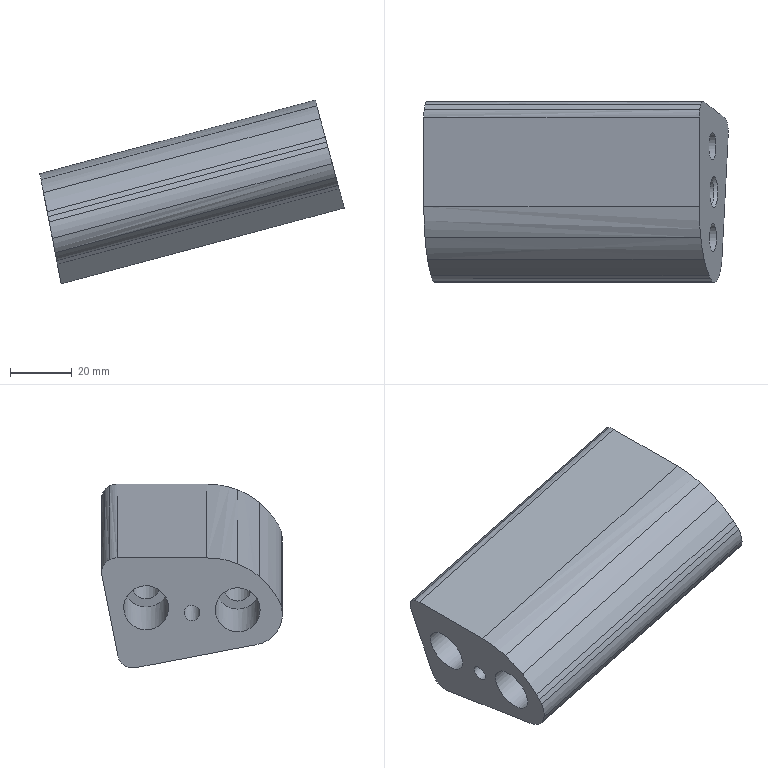Part | NX | features solid 2 | 1 solid | 31 faces | box 98.643 x 58.579 x 59.607 mm | volume 135213 mm3 | spline 16 | plane 8 | cylinder 6 | cone 1 | commonest cylinder face diameters 9.007 x2 14.508 x2 5.1 x1 8 x1
STEP:
#1=CARTESIAN_POINT('',(816.535,-85.556,-16.752));
#2=VERTEX_POINT('',#1);
#3=CARTESIAN_POINT('',(815.148,-85.584,-9.614));
#4=DIRECTION('',(0.9816,0.0002628,0.1908));
#5=DIRECTION('',(0.1908,0.003761,-0.9816));
#6=AXIS2_PLACEMENT_3D('',#3,#4,#5);
#7=ELLIPSE('',#6,7.272,7.254);
#8=EDGE_CURVE('',#2,#2,#7,.T.);
#9=ORIENTED_EDGE('',*,*,#8,.T.);
#10=EDGE_LOOP('',(#9));
#11=FACE_BOUND('',#10,.T.);
#12=CARTESIAN_POINT('',(816.396,-55.874,-16.077));
#13=VERTEX_POINT('',#12);
#14=CARTESIAN_POINT('',(815.009,-55.901,-8.939));
#15=DIRECTION('',(0.9816,0.0002628,0.1908));
#16=DIRECTION('',(0.1908,0.003761,-0.9816));
#17=AXIS2_PLACEMENT_3D('',#14,#15,#16);
#18=ELLIPSE('',#17,7.272,7.254);
#19=EDGE_CURVE('',#13,#13,#18,.T.);
#20=ORIENTED_EDGE('',*,*,#19,.T.);
#21=EDGE_LOOP('',(#20));
#22=FACE_BOUND('',#21,.T.);
#23=CARTESIAN_POINT('',(811.973,-44.117,6.663));
#24=VERTEX_POINT('',#23);
#25=CARTESIAN_POINT('',(811.863,-46.498,7.229));
#26=VERTEX_POINT('',#25);
#27=CARTESIAN_POINT('',(811.973,-44.117,6.663));
#28=CARTESIAN_POINT('',(811.9,-44.854,7.038));
#29=CARTESIAN_POINT('',(811.863,-45.668,7.229));
#30=CARTESIAN_POINT('',(811.863,-46.498,7.229));
#31=B_SPLINE_CURVE_WITH_KNOTS('',3,(#27,#28,#29,#30),.UNSPECIFIED.,.F.,.F.,(4,4),(0.,0.002457),.UNSPECIFIED.);
#32=EDGE_CURVE('',#24,#26,#31,.T.);
#33=ORIENTED_EDGE('',*,*,#32,.F.);
#34=CARTESIAN_POINT('',(812.277,-42.305,5.095));
#35=VERTEX_POINT('',#34);
#36=CARTESIAN_POINT('',(812.277,-42.305,5.095));
#37=CARTESIAN_POINT('',(812.148,-42.767,5.759));
#38=CARTESIAN_POINT('',(812.045,-43.389,6.293));
#39=CARTESIAN_POINT('',(811.973,-44.117,6.663));
#40=B_SPLINE_CURVE_WITH_KNOTS('',3,(#36,#37,#38,#39),.UNSPECIFIED.,.F.,.F.,(4,4),(0.,0.002422),.UNSPECIFIED.);
#41=EDGE_CURVE('',#35,#24,#40,.T.);
#42=ORIENTED_EDGE('',*,*,#41,.F.);
#43=CARTESIAN_POINT('',(812.6,-41.584,3.431));
#44=VERTEX_POINT('',#43);
#45=CARTESIAN_POINT('',(812.6,-41.584,3.431));
#46=CARTESIAN_POINT('',(812.483,-41.711,4.033));
#47=CARTESIAN_POINT('',(812.376,-41.952,4.587));
#48=CARTESIAN_POINT('',(812.277,-42.305,5.095));
#49=B_SPLINE_CURVE_WITH_KNOTS('',3,(#45,#46,#47,#48),.UNSPECIFIED.,.F.,.F.,(4,4),(0.,0.001842),.UNSPECIFIED.);
#50=EDGE_CURVE('',#44,#35,#49,.T.);
#51=ORIENTED_EDGE('',*,*,#50,.F.);
#52=CARTESIAN_POINT('',(812.953,-41.572,1.616));
#53=VERTEX_POINT('',#52);
#54=CARTESIAN_POINT('',(812.953,-41.572,1.616));
#55=CARTESIAN_POINT('',(812.835,-41.454,2.222));
#56=CARTESIAN_POINT('',(812.718,-41.457,2.827));
#57=CARTESIAN_POINT('',(812.6,-41.584,3.431));
#58=B_SPLINE_CURVE_WITH_KNOTS('',3,(#54,#55,#56,#57),.UNSPECIFIED.,.F.,.F.,(4,4),(0.,0.001849),.UNSPECIFIED.);
#59=EDGE_CURVE('',#53,#44,#58,.T.);
#60=ORIENTED_EDGE('',*,*,#59,.F.);
#61=CARTESIAN_POINT('',(814.349,-42.975,-5.566));
#62=VERTEX_POINT('',#61);
#63=CARTESIAN_POINT('',(814.349,-42.975,-5.566));
#64=CARTESIAN_POINT('',(813.884,-42.505,-3.172));
#65=CARTESIAN_POINT('',(813.419,-42.037,-0.7784));
#66=CARTESIAN_POINT('',(812.953,-41.572,1.616));
#67=B_SPLINE_CURVE_WITH_KNOTS('',3,(#63,#64,#65,#66),.UNSPECIFIED.,.F.,.F.,(4,4),(0.,0.007449),.UNSPECIFIED.);
#68=EDGE_CURVE('',#62,#53,#67,.T.);
#69=ORIENTED_EDGE('',*,*,#68,.F.);
#70=CARTESIAN_POINT('',(815.759,-44.406,-12.814));
#71=VERTEX_POINT('',#70);
#72=CARTESIAN_POINT('',(815.759,-44.406,-12.814));
#73=CARTESIAN_POINT('',(815.289,-43.926,-10.398));
#74=CARTESIAN_POINT('',(814.819,-43.45,-7.982));
#75=CARTESIAN_POINT('',(814.349,-42.975,-5.566));
#76=B_SPLINE_CURVE_WITH_KNOTS('',3,(#72,#73,#74,#75),.UNSPECIFIED.,.F.,.F.,(4,4),(0.,0.007522),.UNSPECIFIED.);
#77=EDGE_CURVE('',#71,#62,#76,.T.);
#78=ORIENTED_EDGE('',*,*,#77,.F.);
#79=CARTESIAN_POINT('',(818.03,-46.723,-24.494));
#80=VERTEX_POINT('',#79);
#81=CARTESIAN_POINT('',(813.97,-42.581,-3.616));
#82=DIRECTION('',(0.1873,-0.1911,-0.9635));
#83=VECTOR('',#82,1000.);
#84=LINE('',#81,#83);
#85=EDGE_CURVE('',#71,#80,#84,.T.);
#86=ORIENTED_EDGE('',*,*,#85,.T.);
#87=CARTESIAN_POINT('',(818.785,-52.586,-28.373));
#88=VERTEX_POINT('',#87);
#89=CARTESIAN_POINT('',(818.785,-52.586,-28.373));
#90=CARTESIAN_POINT('',(818.833,-51.29,-28.621));
#91=CARTESIAN_POINT('',(818.723,-48.542,-28.06));
#92=CARTESIAN_POINT('',(818.277,-46.975,-25.766));
#93=CARTESIAN_POINT('',(818.03,-46.723,-24.494));
#94=B_SPLINE_CURVE_WITH_KNOTS('',3,(#89,#90,#91,#92,#93),.UNSPECIFIED.,.F.,.F.,(4,1,4),(0.,0.003905,0.007811),.UNSPECIFIED.);
#95=EDGE_CURVE('',#88,#80,#94,.T.);
#96=ORIENTED_EDGE('',*,*,#95,.F.);
#97=CARTESIAN_POINT('',(817.556,-85.892,-22.005));
#98=VERTEX_POINT('',#97);
#99=CARTESIAN_POINT('',(826.533,157.396,-68.523));
#100=DIRECTION('',(0.03622,0.9816,-0.1877));
#101=VECTOR('',#100,1000.);
#102=LINE('',#99,#101);
#103=EDGE_CURVE('',#98,#88,#102,.T.);
#104=ORIENTED_EDGE('',*,*,#103,.F.);
#105=CARTESIAN_POINT('',(817.343,-91.803,-20.901));
#106=VERTEX_POINT('',#105);
#107=CARTESIAN_POINT('',(817.343,-91.803,-20.901));
#108=CARTESIAN_POINT('',(817.413,-89.831,-21.261));
#109=CARTESIAN_POINT('',(817.484,-87.86,-21.628));
#110=CARTESIAN_POINT('',(817.556,-85.892,-22.005));
#111=B_SPLINE_CURVE_WITH_KNOTS('',3,(#107,#108,#109,#110),.UNSPECIFIED.,.F.,.F.,(4,4),(0.,0.006017),.UNSPECIFIED.);
#112=EDGE_CURVE('',#106,#98,#111,.T.);
#113=ORIENTED_EDGE('',*,*,#112,.F.);
#114=CARTESIAN_POINT('',(816.845,-96.945,-18.332));
#115=VERTEX_POINT('',#114);
#116=CARTESIAN_POINT('',(816.845,-96.945,-18.332));
#117=CARTESIAN_POINT('',(817.103,-95.518,-19.658));
#118=CARTESIAN_POINT('',(817.276,-93.734,-20.549));
#119=CARTESIAN_POINT('',(817.343,-91.803,-20.901));
#120=B_SPLINE_CURVE_WITH_KNOTS('',3,(#116,#117,#118,#119),.UNSPECIFIED.,.F.,.F.,(4,4),(0.,0.005811),.UNSPECIFIED.);
#121=EDGE_CURVE('',#115,#106,#120,.T.);
#122=ORIENTED_EDGE('',*,*,#121,.F.);
#123=CARTESIAN_POINT('',(815.948,-99.734,-13.713));
#124=VERTEX_POINT('',#123);
#125=CARTESIAN_POINT('',(815.948,-99.734,-13.713));
#126=CARTESIAN_POINT('',(816.292,-99.26,-15.479));
#127=CARTESIAN_POINT('',(816.602,-98.295,-17.076));
#128=CARTESIAN_POINT('',(816.845,-96.945,-18.332));
#129=B_SPLINE_CURVE_WITH_KNOTS('',3,(#125,#126,#127,#128),.UNSPECIFIED.,.F.,.F.,(4,4),(0.,0.005502),.UNSPECIFIED.);
#130=EDGE_CURVE('',#124,#115,#129,.T.);
#131=ORIENTED_EDGE('',*,*,#130,.F.);
#132=CARTESIAN_POINT('',(814.903,-99.633,-8.337));
#133=VERTEX_POINT('',#132);
#134=CARTESIAN_POINT('',(815.948,-99.734,-13.713));
#135=CARTESIAN_POINT('',(815.605,-100.208,-11.945));
#136=CARTESIAN_POINT('',(815.244,-100.172,-10.087));
#137=CARTESIAN_POINT('',(814.903,-99.633,-8.337));
#138=B_SPLINE_CURVE_WITH_KNOTS('',3,(#134,#135,#136,#137),.UNSPECIFIED.,.F.,.F.,(4,4),(0.,0.00551),.UNSPECIFIED.);
#139=EDGE_CURVE('',#124,#133,#138,.T.);
#140=ORIENTED_EDGE('',*,*,#139,.T.);
#141=CARTESIAN_POINT('',(814.571,-98.902,-6.628));
#142=VERTEX_POINT('',#141);
#143=CARTESIAN_POINT('',(814.571,-98.902,-6.628));
#144=CARTESIAN_POINT('',(814.677,-99.207,-7.173));
#145=CARTESIAN_POINT('',(814.788,-99.451,-7.742));
#146=CARTESIAN_POINT('',(814.903,-99.633,-8.337));
#147=B_SPLINE_CURVE_WITH_KNOTS('',3,(#143,#144,#145,#146),.UNSPECIFIED.,.F.,.F.,(4,4),(0.,0.001887),.UNSPECIFIED.);
#148=EDGE_CURVE('',#142,#133,#147,.T.);
#149=ORIENTED_EDGE('',*,*,#148,.F.);
#150=CARTESIAN_POINT('',(814.258,-97.948,-5.022));
#151=VERTEX_POINT('',#150);
#152=CARTESIAN_POINT('',(814.258,-97.948,-5.022));
#153=CARTESIAN_POINT('',(814.361,-98.28,-5.549));
#154=CARTESIAN_POINT('',(814.465,-98.598,-6.085));
#155=CARTESIAN_POINT('',(814.571,-98.902,-6.628));
#156=B_SPLINE_CURVE_WITH_KNOTS('',3,(#152,#153,#154,#155),.UNSPECIFIED.,.F.,.F.,(4,4),(0.,0.001895),.UNSPECIFIED.);
#157=EDGE_CURVE('',#151,#142,#156,.T.);
#158=ORIENTED_EDGE('',*,*,#157,.F.);
#159=CARTESIAN_POINT('',(813.062,-92.585,1.127));
#160=VERTEX_POINT('',#159);
#161=CARTESIAN_POINT('',(813.062,-92.585,1.127));
#162=CARTESIAN_POINT('',(813.407,-94.699,-0.6484));
#163=CARTESIAN_POINT('',(813.807,-96.484,-2.701));
#164=CARTESIAN_POINT('',(814.258,-97.948,-5.022));
#165=B_SPLINE_CURVE_WITH_KNOTS('',3,(#161,#162,#163,#164),.UNSPECIFIED.,.F.,.F.,(4,4),(0.,0.008246),.UNSPECIFIED.);
#166=EDGE_CURVE('',#160,#151,#165,.T.);
#167=ORIENTED_EDGE('',*,*,#166,.F.);
#168=CARTESIAN_POINT('',(812.247,-85.562,5.309));
#169=VERTEX_POINT('',#168);
#170=CARTESIAN_POINT('',(812.247,-85.562,5.309));
#171=CARTESIAN_POINT('',(812.446,-88.136,4.29));
#172=CARTESIAN_POINT('',(812.717,-90.477,2.898));
#173=CARTESIAN_POINT('',(813.062,-92.585,1.127));
#174=B_SPLINE_CURVE_WITH_KNOTS('',3,(#170,#171,#172,#173),.UNSPECIFIED.,.F.,.F.,(4,4),(0.,0.008214),.UNSPECIFIED.);
#175=EDGE_CURVE('',#169,#160,#174,.T.);
#176=ORIENTED_EDGE('',*,*,#175,.F.);
#177=CARTESIAN_POINT('',(811.874,-75.541,7.214));
#178=VERTEX_POINT('',#177);
#179=CARTESIAN_POINT('',(811.874,-75.541,7.214));
#180=CARTESIAN_POINT('',(811.875,-79.006,7.212));
#181=CARTESIAN_POINT('',(811.999,-82.348,6.581));
#182=CARTESIAN_POINT('',(812.247,-85.562,5.309));
#183=B_SPLINE_CURVE_WITH_KNOTS('',3,(#179,#180,#181,#182),.UNSPECIFIED.,.F.,.F.,(4,4),(0.,0.01021),.UNSPECIFIED.);
#184=EDGE_CURVE('',#178,#169,#183,.T.);
#185=ORIENTED_EDGE('',*,*,#184,.F.);
#186=CARTESIAN_POINT('',(811.874,-75.571,7.214));
#187=DIRECTION('',(-0.0003677,1.,0.000514));
#188=VECTOR('',#187,1000.);
#189=LINE('',#186,#188);
#190=EDGE_CURVE('',#178,#26,#189,.T.);
#191=ORIENTED_EDGE('',*,*,#190,.T.);
#192=EDGE_LOOP('',(#33,#42,#51,#60,#69,#78,#86,#96,#104,#113,#122,#131,#140,#149,#158,#167,#176,#185,#191));
#193=FACE_BOUND('',#192,.T.);
#194=CARTESIAN_POINT('',(814.852,-70.813,-8.111));
#195=VERTEX_POINT('',#194);
#196=CARTESIAN_POINT('',(815.339,-70.804,-10.62));
#197=DIRECTION('',(0.9816,0.0002628,0.1908));
#198=DIRECTION('',(-0.1908,-0.003761,0.9816));
#199=AXIS2_PLACEMENT_3D('',#196,#197,#198);
#200=ELLIPSE('',#199,2.556,2.55);
#201=EDGE_CURVE('',#195,#195,#200,.F.);
#202=ORIENTED_EDGE('',*,*,#201,.F.);
#203=EDGE_LOOP('',(#202));
#204=FACE_BOUND('',#203,.T.);
#205=CARTESIAN_POINT('',(825.905,158.037,-65.289));
#206=DIRECTION('',(0.9816,0.0002628,0.1908));
#207=DIRECTION('',(-0.1908,0.001526,0.9816));
#208=AXIS2_PLACEMENT_3D('',#205,#206,#207);
#209=PLANE('',#208);
#210=ADVANCED_FACE('',(#11,#22,#193,#204),#209,.F.);
#211=CARTESIAN_POINT('',(907.109,-70.804,8.793));
#212=VERTEX_POINT('',#211);
#213=CARTESIAN_POINT('',(905.814,-70.804,13.623));
#214=DIRECTION('',(0.9659,-0.000000134,0.2588));
#215=DIRECTION('',(0.2588,0.,-0.9659));
#216=AXIS2_PLACEMENT_3D('',#213,#214,#215);
#217=CIRCLE('',#216,5.);
#218=EDGE_CURVE('',#212,#212,#217,.F.);
#219=ORIENTED_EDGE('',*,*,#218,.T.);
#220=EDGE_LOOP('',(#219));
#221=FACE_BOUND('',#220,.T.);
#222=CARTESIAN_POINT('',(904.207,-55.901,19.624));
#223=VERTEX_POINT('',#222);
#224=CARTESIAN_POINT('',(905.372,-55.901,15.274));
#225=DIRECTION('',(0.9659,-0.000000134,0.2588));
#226=DIRECTION('',(-0.2588,0.,0.9659));
#227=AXIS2_PLACEMENT_3D('',#224,#225,#226);
#228=CIRCLE('',#227,4.503);
#229=EDGE_CURVE('',#223,#223,#228,.T.);
#230=ORIENTED_EDGE('',*,*,#229,.F.);
#231=EDGE_LOOP('',(#230));
#232=FACE_BOUND('',#231,.T.);
#233=CARTESIAN_POINT('',(906.391,-44.406,11.471));
#234=VERTEX_POINT('',#233);
#235=CARTESIAN_POINT('',(904.485,-42.975,18.586));
#236=VERTEX_POINT('',#235);
#237=CARTESIAN_POINT('',(906.391,-44.406,11.471));
#238=CARTESIAN_POINT('',(905.756,-43.926,13.842));
#239=CARTESIAN_POINT('',(905.12,-43.45,16.214));
#240=CARTESIAN_POINT('',(904.485,-42.975,18.586));
#241=B_SPLINE_CURVE_WITH_KNOTS('',3,(#237,#238,#239,#240),.UNSPECIFIED.,.F.,.F.,(4,4),(0.,0.007504),.UNSPECIFIED.);
#242=EDGE_CURVE('',#234,#236,#241,.T.);
#243=ORIENTED_EDGE('',*,*,#242,.T.);
#244=CARTESIAN_POINT('',(902.596,-41.572,25.636));
#245=VERTEX_POINT('',#244);
#246=CARTESIAN_POINT('',(902.596,-41.572,25.636));
#247=CARTESIAN_POINT('',(903.225,-42.037,23.285));
#248=CARTESIAN_POINT('',(903.855,-42.505,20.935));
#249=CARTESIAN_POINT('',(904.485,-42.975,18.586));
#250=B_SPLINE_CURVE_WITH_KNOTS('',3,(#246,#247,#248,#249),.UNSPECIFIED.,.F.,.F.,(4,4),(0.,0.007432),.UNSPECIFIED.);
#251=EDGE_CURVE('',#245,#236,#250,.T.);
#252=ORIENTED_EDGE('',*,*,#251,.F.);
#253=CARTESIAN_POINT('',(902.118,-41.584,27.417));
#254=VERTEX_POINT('',#253);
#255=CARTESIAN_POINT('',(902.118,-41.584,27.417));
#256=CARTESIAN_POINT('',(902.277,-41.457,26.824));
#257=CARTESIAN_POINT('',(902.436,-41.454,26.23));
#258=CARTESIAN_POINT('',(902.596,-41.572,25.636));
#259=B_SPLINE_CURVE_WITH_KNOTS('',3,(#255,#256,#257,#258),.UNSPECIFIED.,.F.,.F.,(4,4),(0.,0.001844),.UNSPECIFIED.);
#260=EDGE_CURVE('',#254,#245,#259,.T.);
#261=ORIENTED_EDGE('',*,*,#260,.F.);
#262=CARTESIAN_POINT('',(901.681,-42.305,29.051));
#263=VERTEX_POINT('',#262);
#264=CARTESIAN_POINT('',(901.681,-42.305,29.051));
#265=CARTESIAN_POINT('',(901.814,-41.952,28.553));
#266=CARTESIAN_POINT('',(901.96,-41.711,28.008));
#267=CARTESIAN_POINT('',(902.118,-41.584,27.417));
#268=B_SPLINE_CURVE_WITH_KNOTS('',3,(#264,#265,#266,#267),.UNSPECIFIED.,.F.,.F.,(4,4),(0.,0.001839),.UNSPECIFIED.);
#269=EDGE_CURVE('',#263,#254,#268,.T.);
#270=ORIENTED_EDGE('',*,*,#269,.F.);
#271=CARTESIAN_POINT('',(901.268,-44.117,30.589));
#272=VERTEX_POINT('',#271);
#273=CARTESIAN_POINT('',(901.268,-44.117,30.589));
#274=CARTESIAN_POINT('',(901.365,-43.39,30.227));
#275=CARTESIAN_POINT('',(901.506,-42.767,29.703));
#276=CARTESIAN_POINT('',(901.681,-42.305,29.051));
#277=B_SPLINE_CURVE_WITH_KNOTS('',3,(#273,#274,#275,#276),.UNSPECIFIED.,.F.,.F.,(4,4),(0.,0.00242),.UNSPECIFIED.);
#278=EDGE_CURVE('',#272,#263,#277,.T.);
#279=ORIENTED_EDGE('',*,*,#278,.F.);
#280=CARTESIAN_POINT('',(901.119,-46.498,31.145));
#281=VERTEX_POINT('',#280);
#282=CARTESIAN_POINT('',(901.119,-46.498,31.145));
#283=CARTESIAN_POINT('',(901.119,-45.668,31.146));
#284=CARTESIAN_POINT('',(901.17,-44.855,30.957));
#285=CARTESIAN_POINT('',(901.268,-44.117,30.589));
#286=B_SPLINE_CURVE_WITH_KNOTS('',3,(#282,#283,#284,#285),.UNSPECIFIED.,.F.,.F.,(4,4),(0.,0.002456),.UNSPECIFIED.);
#287=EDGE_CURVE('',#281,#272,#286,.T.);
#288=ORIENTED_EDGE('',*,*,#287,.F.);
#289=CARTESIAN_POINT('',(901.124,-75.541,31.128));
#290=VERTEX_POINT('',#289);
#291=CARTESIAN_POINT('',(901.124,-75.541,31.128));
#292=DIRECTION('',(-0.000153,1.,0.0005715));
#293=VECTOR('',#292,1000.);
#294=LINE('',#291,#293);
#295=EDGE_CURVE('',#290,#281,#294,.T.);
#296=ORIENTED_EDGE('',*,*,#295,.F.);
#297=CARTESIAN_POINT('',(901.625,-85.563,29.257));
#298=VERTEX_POINT('',#297);
#299=CARTESIAN_POINT('',(901.124,-75.541,31.128));
#300=CARTESIAN_POINT('',(901.124,-79.006,31.126));
#301=CARTESIAN_POINT('',(901.29,-82.347,30.507));
#302=CARTESIAN_POINT('',(901.625,-85.563,29.257));
#303=B_SPLINE_CURVE_WITH_KNOTS('',3,(#299,#300,#301,#302),.UNSPECIFIED.,.F.,.F.,(4,4),(0.,0.01021),.UNSPECIFIED.);
#304=EDGE_CURVE('',#290,#298,#303,.T.);
#305=ORIENTED_EDGE('',*,*,#304,.T.);
#306=CARTESIAN_POINT('',(902.725,-92.585,25.152));
#307=VERTEX_POINT('',#306);
#308=CARTESIAN_POINT('',(902.725,-92.585,25.152));
#309=CARTESIAN_POINT('',(902.259,-90.477,26.891));
#310=CARTESIAN_POINT('',(901.893,-88.135,28.258));
#311=CARTESIAN_POINT('',(901.625,-85.563,29.257));
#312=B_SPLINE_CURVE_WITH_KNOTS('',3,(#308,#309,#310,#311),.UNSPECIFIED.,.F.,.F.,(4,4),(0.,0.008209),.UNSPECIFIED.);
#313=EDGE_CURVE('',#307,#298,#312,.T.);
#314=ORIENTED_EDGE('',*,*,#313,.F.);
#315=CARTESIAN_POINT('',(904.343,-97.948,19.116));
#316=VERTEX_POINT('',#315);
#317=CARTESIAN_POINT('',(904.343,-97.948,19.116));
#318=CARTESIAN_POINT('',(903.732,-96.483,21.396));
#319=CARTESIAN_POINT('',(903.192,-94.698,23.41));
#320=CARTESIAN_POINT('',(902.725,-92.585,25.152));
#321=B_SPLINE_CURVE_WITH_KNOTS('',3,(#317,#318,#319,#320),.UNSPECIFIED.,.F.,.F.,(4,4),(0.,0.008235),.UNSPECIFIED.);
#322=EDGE_CURVE('',#316,#307,#321,.T.);
#323=ORIENTED_EDGE('',*,*,#322,.F.);
#324=CARTESIAN_POINT('',(904.765,-98.902,17.539));
#325=VERTEX_POINT('',#324);
#326=CARTESIAN_POINT('',(904.765,-98.902,17.539));
#327=CARTESIAN_POINT('',(904.622,-98.598,18.073));
#328=CARTESIAN_POINT('',(904.481,-98.28,18.598));
#329=CARTESIAN_POINT('',(904.343,-97.948,19.116));
#330=B_SPLINE_CURVE_WITH_KNOTS('',3,(#326,#327,#328,#329),.UNSPECIFIED.,.F.,.F.,(4,4),(0.,0.001891),.UNSPECIFIED.);
#331=EDGE_CURVE('',#325,#316,#330,.T.);
#332=ORIENTED_EDGE('',*,*,#331,.F.);
#333=CARTESIAN_POINT('',(905.214,-99.633,15.862));
#334=VERTEX_POINT('',#333);
#335=CARTESIAN_POINT('',(905.214,-99.633,15.862));
#336=CARTESIAN_POINT('',(905.058,-99.451,16.446));
#337=CARTESIAN_POINT('',(904.908,-99.207,17.005));
#338=CARTESIAN_POINT('',(904.765,-98.902,17.539));
#339=B_SPLINE_CURVE_WITH_KNOTS('',3,(#335,#336,#337,#338),.UNSPECIFIED.,.F.,.F.,(4,4),(0.,0.001884),.UNSPECIFIED.);
#340=EDGE_CURVE('',#334,#325,#339,.T.);
#341=ORIENTED_EDGE('',*,*,#340,.F.);
#342=CARTESIAN_POINT('',(906.629,-99.734,10.584));
#343=VERTEX_POINT('',#342);
#344=CARTESIAN_POINT('',(906.629,-99.734,10.584));
#345=CARTESIAN_POINT('',(906.163,-100.208,12.32));
#346=CARTESIAN_POINT('',(905.675,-100.172,14.144));
#347=CARTESIAN_POINT('',(905.214,-99.633,15.862));
#348=B_SPLINE_CURVE_WITH_KNOTS('',3,(#344,#345,#346,#347),.UNSPECIFIED.,.F.,.F.,(4,4),(0.,0.005497),.UNSPECIFIED.);
#349=EDGE_CURVE('',#343,#334,#348,.T.);
#350=ORIENTED_EDGE('',*,*,#349,.F.);
#351=CARTESIAN_POINT('',(907.843,-96.945,6.051));
#352=VERTEX_POINT('',#351);
#353=CARTESIAN_POINT('',(907.843,-96.945,6.051));
#354=CARTESIAN_POINT('',(907.513,-98.295,7.283));
#355=CARTESIAN_POINT('',(907.093,-99.26,8.85));
#356=CARTESIAN_POINT('',(906.629,-99.734,10.584));
#357=B_SPLINE_CURVE_WITH_KNOTS('',3,(#353,#354,#355,#356),.UNSPECIFIED.,.F.,.F.,(4,4),(0.,0.005492),.UNSPECIFIED.);
#358=EDGE_CURVE('',#352,#343,#357,.T.);
#359=ORIENTED_EDGE('',*,*,#358,.F.);
#360=CARTESIAN_POINT('',(908.519,-91.803,3.529));
#361=VERTEX_POINT('',#360);
#362=CARTESIAN_POINT('',(907.843,-96.945,6.051));
#363=CARTESIAN_POINT('',(908.192,-95.517,4.748));
#364=CARTESIAN_POINT('',(908.427,-93.734,3.874));
#365=CARTESIAN_POINT('',(908.519,-91.803,3.529));
#366=B_SPLINE_CURVE_WITH_KNOTS('',3,(#362,#363,#364,#365),.UNSPECIFIED.,.F.,.F.,(4,4),(0.,0.005808),.UNSPECIFIED.);
#367=EDGE_CURVE('',#352,#361,#366,.T.);
#368=ORIENTED_EDGE('',*,*,#367,.T.);
#369=CARTESIAN_POINT('',(908.809,-85.892,2.446));
#370=VERTEX_POINT('',#369);
#371=CARTESIAN_POINT('',(908.809,-85.892,2.446));
#372=CARTESIAN_POINT('',(908.71,-87.86,2.816));
#373=CARTESIAN_POINT('',(908.613,-89.831,3.177));
#374=CARTESIAN_POINT('',(908.519,-91.803,3.529));
#375=B_SPLINE_CURVE_WITH_KNOTS('',3,(#371,#372,#373,#374),.UNSPECIFIED.,.F.,.F.,(4,4),(0.,0.006016),.UNSPECIFIED.);
#376=EDGE_CURVE('',#370,#361,#375,.T.);
#377=ORIENTED_EDGE('',*,*,#376,.F.);
#378=CARTESIAN_POINT('',(910.484,-52.586,-3.803));
#379=VERTEX_POINT('',#378);
#380=CARTESIAN_POINT('',(910.484,-52.586,-3.803));
#381=DIRECTION('',(-0.04935,-0.9817,0.1842));
#382=VECTOR('',#381,1000.);
#383=LINE('',#380,#382);
#384=EDGE_CURVE('',#379,#370,#383,.T.);
#385=ORIENTED_EDGE('',*,*,#384,.F.);
#386=CARTESIAN_POINT('',(909.463,-46.723,0.005641));
#387=VERTEX_POINT('',#386);
#388=CARTESIAN_POINT('',(909.463,-46.723,0.005641));
#389=CARTESIAN_POINT('',(909.798,-46.976,-1.245));
#390=CARTESIAN_POINT('',(910.401,-48.54,-3.493));
#391=CARTESIAN_POINT('',(910.549,-51.291,-4.046));
#392=CARTESIAN_POINT('',(910.484,-52.586,-3.803));
#393=B_SPLINE_CURVE_WITH_KNOTS('',3,(#388,#389,#390,#391,#392),.UNSPECIFIED.,.F.,.F.,(4,1,4),(0.,0.003902,0.007804),.UNSPECIFIED.);
#394=EDGE_CURVE('',#387,#379,#393,.T.);
#395=ORIENTED_EDGE('',*,*,#394,.F.);
#396=CARTESIAN_POINT('',(906.391,-44.406,11.471));
#397=DIRECTION('',(0.254,-0.1916,-0.948));
#398=VECTOR('',#397,1000.);
#399=LINE('',#396,#398);
#400=EDGE_CURVE('',#234,#387,#399,.T.);
#401=ORIENTED_EDGE('',*,*,#400,.F.);
#402=EDGE_LOOP('',(#243,#252,#261,#270,#279,#288,#296,#305,#314,#323,#332,#341,#350,#359,#368,#377,#385,#395,#401));
#403=FACE_BOUND('',#402,.T.);
#404=CARTESIAN_POINT('',(904.384,-85.584,18.96));
#405=VERTEX_POINT('',#404);
#406=CARTESIAN_POINT('',(905.55,-85.584,14.61));
#407=DIRECTION('',(0.9659,-0.000000134,0.2588));
#408=DIRECTION('',(-0.2588,0.,0.9659));
#409=AXIS2_PLACEMENT_3D('',#406,#407,#408);
#410=CIRCLE('',#409,4.503);
#411=EDGE_CURVE('',#405,#405,#410,.T.);
#412=ORIENTED_EDGE('',*,*,#411,.F.);
#413=EDGE_LOOP('',(#412));
#414=FACE_BOUND('',#413,.T.);
#415=CARTESIAN_POINT('',(1072.245,4.191,-607.503));
#416=DIRECTION('',(0.9659,-0.000000134,0.2588));
#417=DIRECTION('',(-0.2588,0.,0.9659));
#418=AXIS2_PLACEMENT_3D('',#415,#416,#417);
#419=PLANE('',#418);
#420=ADVANCED_FACE('',(#221,#232,#403,#414),#419,.T.);
#421=ORIENTED_EDGE('',*,*,#411,.T.);
#422=EDGE_LOOP('',(#421));
#423=FACE_BOUND('',#422,.T.);
#424=CARTESIAN_POINT('',(843.198,-85.584,-6.76));
#425=VERTEX_POINT('',#424);
#426=CARTESIAN_POINT('',(842.032,-85.584,-2.41));
#427=DIRECTION('',(-0.9659,0.000000134,-0.2588));
#428=DIRECTION('',(0.2588,0.,-0.9659));
#429=AXIS2_PLACEMENT_3D('',#426,#427,#428);
#430=CIRCLE('',#429,4.503);
#431=EDGE_CURVE('',#425,#425,#430,.F.);
#432=ORIENTED_EDGE('',*,*,#431,.F.);
#433=EDGE_LOOP('',(#432));
#434=FACE_BOUND('',#433,.T.);
#435=CARTESIAN_POINT('',(792.77,-85.584,-15.61));
#436=DIRECTION('',(0.9659,-0.000000134,0.2588));
#437=DIRECTION('',(-0.2588,0.,0.9659));
#438=AXIS2_PLACEMENT_3D('',#435,#436,#437);
#439=CYLINDRICAL_SURFACE('',#438,4.503);
#440=ADVANCED_FACE('',(#423,#434),#439,.F.);
#441=CARTESIAN_POINT('',(841.674,-92.705,-1.074));
#442=VERTEX_POINT('',#441);
#443=CARTESIAN_POINT('',(842.032,-85.584,-2.41));
#444=DIRECTION('',(-0.9659,0.000000134,-0.2588));
#445=DIRECTION('',(-0.04935,-0.9817,0.1842));
#446=AXIS2_PLACEMENT_3D('',#443,#444,#445);
#447=CIRCLE('',#446,7.254);
#448=EDGE_CURVE('',#442,#442,#447,.F.);
#449=ORIENTED_EDGE('',*,*,#448,.F.);
#450=EDGE_LOOP('',(#449));
#451=FACE_BOUND('',#450,.T.);
#452=ORIENTED_EDGE('',*,*,#431,.T.);
#453=EDGE_LOOP('',(#452));
#454=FACE_BOUND('',#453,.T.);
#455=CARTESIAN_POINT('',(842.032,-85.584,-2.41));
#456=DIRECTION('',(-0.9659,0.000000134,-0.2588));
#457=DIRECTION('',(0.2588,0.,-0.9659));
#458=AXIS2_PLACEMENT_3D('',#455,#456,#457);
#459=PLANE('',#458);
#460=ADVANCED_FACE('',(#451,#454),#459,.T.);
#461=ORIENTED_EDGE('',*,*,#448,.T.);
#462=EDGE_LOOP('',(#461));
#463=FACE_BOUND('',#462,.T.);
#464=ORIENTED_EDGE('',*,*,#8,.F.);
#465=EDGE_LOOP('',(#464));
#466=FACE_BOUND('',#465,.T.);
#467=CARTESIAN_POINT('',(842.032,-85.584,-2.41));
#468=DIRECTION('',(-0.9659,0.000000134,-0.2588));
#469=DIRECTION('',(0.2588,0.,-0.9659));
#470=AXIS2_PLACEMENT_3D('',#467,#468,#469);
#471=CYLINDRICAL_SURFACE('',#470,7.254);
#472=ADVANCED_FACE('',(#463,#466),#471,.F.);
#473=CARTESIAN_POINT('',(942.8,-46.498,42.313));
#474=DIRECTION('',(-0.9659,0.000000134,-0.2588));
#475=VECTOR('',#474,1000.);
#476=LINE('',#473,#475);
#477=EDGE_CURVE('',#26,#281,#476,.F.);
#478=ORIENTED_EDGE('',*,*,#477,.F.);
#479=ORIENTED_EDGE('',*,*,#190,.F.);
#480=CARTESIAN_POINT('',(942.866,-75.541,42.313));
#481=DIRECTION('',(-0.9659,0.000000134,-0.2588));
#482=VECTOR('',#481,1000.);
#483=LINE('',#480,#482);
#484=EDGE_CURVE('',#178,#290,#483,.F.);
#485=ORIENTED_EDGE('',*,*,#484,.T.);
#486=ORIENTED_EDGE('',*,*,#295,.T.);
#487=EDGE_LOOP('',(#478,#479,#485,#486));
#488=FACE_BOUND('',#487,.T.);
#489=CARTESIAN_POINT('',(942.866,-75.541,42.313));
#490=DIRECTION('',(-0.2588,-0.0005916,0.9659));
#491=DIRECTION('',(-0.9659,0.,-0.2588));
#492=AXIS2_PLACEMENT_3D('',#489,#490,#491);
#493=PLANE('',#492);
#494=ADVANCED_FACE('',(#488),#493,.T.);
#495=CARTESIAN_POINT('',(944.834,-41.584,38.862));
#496=DIRECTION('',(-0.9659,0.000000134,-0.2588));
#497=VECTOR('',#496,1000.);
#498=LINE('',#495,#497);
#499=EDGE_CURVE('',#44,#254,#498,.F.);
#500=ORIENTED_EDGE('',*,*,#499,.F.);
#501=ORIENTED_EDGE('',*,*,#50,.T.);
#502=CARTESIAN_POINT('',(943.956,-42.305,40.379));
#503=DIRECTION('',(-0.9659,0.000000134,-0.2588));
#504=VECTOR('',#503,1000.);
#505=LINE('',#502,#504);
#506=EDGE_CURVE('',#35,#263,#505,.F.);
#507=ORIENTED_EDGE('',*,*,#506,.T.);
#508=ORIENTED_EDGE('',*,*,#269,.T.);
#509=EDGE_LOOP('',(#500,#501,#507,#508));
#510=FACE_BOUND('',#509,.T.);
#511=CARTESIAN_POINT('',(902.22,-42.305,29.195));
#512=CARTESIAN_POINT('',(811.183,-42.305,4.802));
#513=CARTESIAN_POINT('',(902.494,-41.956,28.741));
#514=CARTESIAN_POINT('',(811.457,-41.956,4.347));
#515=CARTESIAN_POINT('',(902.793,-41.709,28.223));
#516=CARTESIAN_POINT('',(811.756,-41.709,3.829));
#517=CARTESIAN_POINT('',(903.097,-41.584,27.679));
#518=CARTESIAN_POINT('',(812.061,-41.584,3.286));
#519=B_SPLINE_SURFACE_WITH_KNOTS('',3,1,((#511,#512),(#513,#514),(#515,#516),(#517,#518)),.SURF_OF_LINEAR_EXTRUSION.,.F.,.F.,.F.,(4,4),(2,2),(6.091,6.476),(0.,1.),.PIECEWISE_BEZIER_KNOTS.);
#520=ADVANCED_FACE('',(#510),#519,.T.);
#521=ORIENTED_EDGE('',*,*,#506,.F.);
#522=ORIENTED_EDGE('',*,*,#41,.T.);
#523=CARTESIAN_POINT('',(943.104,-44.117,41.799));
#524=DIRECTION('',(-0.9659,0.000000134,-0.2588));
#525=VECTOR('',#524,1000.);
#526=LINE('',#523,#525);
#527=EDGE_CURVE('',#24,#272,#526,.F.);
#528=ORIENTED_EDGE('',*,*,#527,.T.);
#529=ORIENTED_EDGE('',*,*,#278,.T.);
#530=EDGE_LOOP('',(#521,#522,#528,#529));
#531=FACE_BOUND('',#530,.T.);
#532=CARTESIAN_POINT('',(901.807,-44.117,30.734));
#533=CARTESIAN_POINT('',(810.886,-44.117,6.371));
#534=CARTESIAN_POINT('',(902.008,-43.388,30.398));
#535=CARTESIAN_POINT('',(811.086,-43.388,6.035));
#536=CARTESIAN_POINT('',(902.304,-42.76,29.905));
#537=CARTESIAN_POINT('',(811.382,-42.76,5.542));
#538=CARTESIAN_POINT('',(902.66,-42.305,29.313));
#539=CARTESIAN_POINT('',(811.738,-42.305,4.951));
#540=B_SPLINE_SURFACE_WITH_KNOTS('',3,1,((#532,#533),(#534,#535),(#536,#537),(#538,#539)),.SURF_OF_LINEAR_EXTRUSION.,.F.,.F.,.F.,(4,4),(2,2),(0.7564,1.252),(0.,1.),.PIECEWISE_BEZIER_KNOTS.);
#541=ADVANCED_FACE('',(#531),#540,.T.);
#542=ORIENTED_EDGE('',*,*,#527,.F.);
#543=ORIENTED_EDGE('',*,*,#32,.T.);
#544=ORIENTED_EDGE('',*,*,#477,.T.);
#545=ORIENTED_EDGE('',*,*,#287,.T.);
#546=EDGE_LOOP('',(#542,#543,#544,#545));
#547=FACE_BOUND('',#546,.T.);
#548=CARTESIAN_POINT('',(901.657,-46.498,31.289));
#549=CARTESIAN_POINT('',(811.132,-46.498,7.033));
#550=CARTESIAN_POINT('',(901.655,-45.671,31.289));
#551=CARTESIAN_POINT('',(811.13,-45.671,7.033));
#552=CARTESIAN_POINT('',(901.761,-44.845,31.111));
#553=CARTESIAN_POINT('',(811.235,-44.845,6.855));
#554=CARTESIAN_POINT('',(901.962,-44.117,30.775));
#555=CARTESIAN_POINT('',(811.436,-44.117,6.519));
#556=B_SPLINE_SURFACE_WITH_KNOTS('',3,1,((#548,#549),(#550,#551),(#552,#553),(#554,#555)),.SURF_OF_LINEAR_EXTRUSION.,.F.,.F.,.F.,(4,4),(2,2),(0.2624,0.7564),(0.,1.),.PIECEWISE_BEZIER_KNOTS.);
#557=ADVANCED_FACE('',(#547),#556,.T.);
#558=ORIENTED_EDGE('',*,*,#484,.F.);
#559=ORIENTED_EDGE('',*,*,#184,.T.);
#560=CARTESIAN_POINT('',(943.927,-85.563,40.592));
#561=DIRECTION('',(-0.9659,0.000000134,-0.2588));
#562=VECTOR('',#561,1000.);
#563=LINE('',#560,#562);
#564=EDGE_CURVE('',#169,#298,#563,.F.);
#565=ORIENTED_EDGE('',*,*,#564,.T.);
#566=ORIENTED_EDGE('',*,*,#304,.F.);
#567=EDGE_LOOP('',(#558,#559,#565,#566));
#568=FACE_BOUND('',#567,.T.);
#569=CARTESIAN_POINT('',(902.724,-85.563,29.552));
#570=CARTESIAN_POINT('',(811.707,-85.562,5.164));
#571=CARTESIAN_POINT('',(902.034,-82.399,30.684));
#572=CARTESIAN_POINT('',(811.017,-82.399,6.296));
#573=CARTESIAN_POINT('',(901.671,-78.971,31.273));
#574=CARTESIAN_POINT('',(810.655,-78.971,6.885));
#575=CARTESIAN_POINT('',(901.663,-75.541,31.273));
#576=CARTESIAN_POINT('',(810.647,-75.541,6.885));
#577=B_SPLINE_SURFACE_WITH_KNOTS('',3,1,((#569,#570),(#571,#572),(#573,#574),(#575,#576)),.SURF_OF_LINEAR_EXTRUSION.,.F.,.F.,.F.,(4,4),(2,2),(6.085,6.481),(0.,1.),.PIECEWISE_BEZIER_KNOTS.);
#578=ADVANCED_FACE('',(#568),#577,.T.);
#579=ORIENTED_EDGE('',*,*,#564,.F.);
#580=ORIENTED_EDGE('',*,*,#175,.T.);
#581=CARTESIAN_POINT('',(946.038,-92.585,36.758));
#582=DIRECTION('',(-0.9659,0.000000134,-0.2588));
#583=VECTOR('',#582,1000.);
#584=LINE('',#581,#583);
#585=EDGE_CURVE('',#160,#307,#584,.F.);
#586=ORIENTED_EDGE('',*,*,#585,.T.);
#587=ORIENTED_EDGE('',*,*,#313,.T.);
#588=EDGE_LOOP('',(#579,#580,#586,#587));
#589=FACE_BOUND('',#588,.T.);
#590=CARTESIAN_POINT('',(904.281,-92.585,25.569));
#591=CARTESIAN_POINT('',(812.518,-92.585,0.9813));
#592=CARTESIAN_POINT('',(903.443,-90.499,27.188));
#593=CARTESIAN_POINT('',(811.679,-90.499,2.6));
#594=CARTESIAN_POINT('',(902.727,-88.118,28.488));
#595=CARTESIAN_POINT('',(810.963,-88.118,3.901));
#596=CARTESIAN_POINT('',(902.169,-85.563,29.403));
#597=CARTESIAN_POINT('',(810.406,-85.562,4.815));
#598=B_SPLINE_SURFACE_WITH_KNOTS('',3,1,((#590,#591),(#592,#593),(#594,#595),(#596,#597)),.SURF_OF_LINEAR_EXTRUSION.,.F.,.F.,.F.,(4,4),(2,2),(6.122,6.445),(0.,1.),.PIECEWISE_BEZIER_KNOTS.);
#599=ADVANCED_FACE('',(#589),#598,.T.);
#600=ORIENTED_EDGE('',*,*,#585,.F.);
#601=ORIENTED_EDGE('',*,*,#166,.T.);
#602=CARTESIAN_POINT('',(948.491,-97.948,30.945));
#603=DIRECTION('',(-0.9659,0.000000134,-0.2588));
#604=VECTOR('',#603,1000.);
#605=LINE('',#602,#604);
#606=EDGE_CURVE('',#151,#316,#605,.F.);
#607=ORIENTED_EDGE('',*,*,#606,.T.);
#608=ORIENTED_EDGE('',*,*,#322,.T.);
#609=EDGE_LOOP('',(#600,#601,#607,#608));
#610=FACE_BOUND('',#609,.T.);
#611=CARTESIAN_POINT('',(905.723,-97.948,19.486));
#612=CARTESIAN_POINT('',(813.713,-97.948,-5.168));
#613=CARTESIAN_POINT('',(904.94,-96.49,21.709));
#614=CARTESIAN_POINT('',(812.93,-96.489,-2.945));
#615=CARTESIAN_POINT('',(904.109,-94.672,23.679));
#616=CARTESIAN_POINT('',(812.099,-94.672,-0.975));
#617=CARTESIAN_POINT('',(903.271,-92.585,25.298));
#618=CARTESIAN_POINT('',(811.261,-92.585,0.6445));
#619=B_SPLINE_SURFACE_WITH_KNOTS('',3,1,((#611,#612),(#613,#614),(#615,#616),(#617,#618)),.SURF_OF_LINEAR_EXTRUSION.,.F.,.F.,.F.,(4,4),(2,2),(6.125,6.441),(0.,1.),.PIECEWISE_BEZIER_KNOTS.);
#620=ADVANCED_FACE('',(#610),#619,.T.);
#621=ORIENTED_EDGE('',*,*,#606,.F.);
#622=ORIENTED_EDGE('',*,*,#157,.T.);
#623=CARTESIAN_POINT('',(949.009,-98.902,29.394));
#624=DIRECTION('',(-0.9659,0.000000134,-0.2588));
#625=VECTOR('',#624,1000.);
#626=LINE('',#623,#625);
#627=EDGE_CURVE('',#142,#325,#626,.F.);
#628=ORIENTED_EDGE('',*,*,#627,.T.);
#629=ORIENTED_EDGE('',*,*,#331,.T.);
#630=EDGE_LOOP('',(#621,#622,#628,#629));
#631=FACE_BOUND('',#630,.T.);
#632=CARTESIAN_POINT('',(905.402,-98.902,17.71));
#633=CARTESIAN_POINT('',(814.029,-98.902,-6.774));
#634=CARTESIAN_POINT('',(905.235,-98.598,18.237));
#635=CARTESIAN_POINT('',(813.862,-98.598,-6.246));
#636=CARTESIAN_POINT('',(905.063,-98.28,18.755));
#637=CARTESIAN_POINT('',(813.689,-98.28,-5.729));
#638=CARTESIAN_POINT('',(904.884,-97.948,19.261));
#639=CARTESIAN_POINT('',(813.511,-97.948,-5.222));
#640=B_SPLINE_SURFACE_WITH_KNOTS('',3,1,((#632,#633),(#634,#635),(#636,#637),(#638,#639)),.SURF_OF_LINEAR_EXTRUSION.,.F.,.F.,.F.,(4,4),(2,2),(6.254,6.312),(0.,1.),.PIECEWISE_BEZIER_KNOTS.);
#641=ADVANCED_FACE('',(#631),#640,.T.);
#642=ORIENTED_EDGE('',*,*,#627,.F.);
#643=ORIENTED_EDGE('',*,*,#148,.T.);
#644=CARTESIAN_POINT('',(949.504,-99.634,27.73));
#645=DIRECTION('',(-0.9659,0.000000134,-0.2588));
#646=VECTOR('',#645,1000.);
#647=LINE('',#644,#646);
#648=EDGE_CURVE('',#133,#334,#647,.F.);
#649=ORIENTED_EDGE('',*,*,#648,.T.);
#650=ORIENTED_EDGE('',*,*,#340,.T.);
#651=EDGE_LOOP('',(#642,#643,#649,#650));
#652=FACE_BOUND('',#651,.T.);
#653=CARTESIAN_POINT('',(905.802,-99.633,16.02));
#654=CARTESIAN_POINT('',(814.361,-99.633,-8.482));
#655=CARTESIAN_POINT('',(905.64,-99.451,16.6));
#656=CARTESIAN_POINT('',(814.199,-99.451,-7.902));
#657=CARTESIAN_POINT('',(905.474,-99.206,17.159));
#658=CARTESIAN_POINT('',(814.033,-99.206,-7.343));
#659=CARTESIAN_POINT('',(905.307,-98.902,17.684));
#660=CARTESIAN_POINT('',(813.866,-98.902,-6.817));
#661=B_SPLINE_SURFACE_WITH_KNOTS('',3,1,((#653,#654),(#655,#656),(#657,#658),(#659,#660)),.SURF_OF_LINEAR_EXTRUSION.,.F.,.F.,.F.,(4,4),(2,2),(6.178,6.389),(0.,1.),.PIECEWISE_BEZIER_KNOTS.);
#662=ADVANCED_FACE('',(#652),#661,.T.);
#663=ORIENTED_EDGE('',*,*,#648,.F.);
#664=ORIENTED_EDGE('',*,*,#139,.F.);
#665=CARTESIAN_POINT('',(950.741,-99.734,22.404));
#666=DIRECTION('',(-0.9659,0.000000134,-0.2588));
#667=VECTOR('',#666,1000.);
#668=LINE('',#665,#667);
#669=EDGE_CURVE('',#124,#343,#668,.F.);
#670=ORIENTED_EDGE('',*,*,#669,.T.);
#671=ORIENTED_EDGE('',*,*,#349,.T.);
#672=EDGE_LOOP('',(#663,#664,#670,#671));
#673=FACE_BOUND('',#672,.T.);
#674=CARTESIAN_POINT('',(907.173,-99.734,10.73));
#675=CARTESIAN_POINT('',(815.4,-99.734,-13.86));
#676=CARTESIAN_POINT('',(906.846,-100.204,12.486));
#677=CARTESIAN_POINT('',(815.073,-100.204,-12.105));
#678=CARTESIAN_POINT('',(906.412,-100.169,14.353));
#679=CARTESIAN_POINT('',(814.639,-100.169,-10.237));
#680=CARTESIAN_POINT('',(905.936,-99.633,16.056));
#681=CARTESIAN_POINT('',(814.163,-99.633,-8.535));
#682=B_SPLINE_SURFACE_WITH_KNOTS('',3,1,((#674,#675),(#676,#677),(#678,#679),(#680,#681)),.SURF_OF_LINEAR_EXTRUSION.,.F.,.F.,.F.,(4,4),(2,2),(6.004,6.562),(0.,1.),.PIECEWISE_BEZIER_KNOTS.);
#683=ADVANCED_FACE('',(#673),#682,.T.);
#684=ORIENTED_EDGE('',*,*,#669,.F.);
#685=ORIENTED_EDGE('',*,*,#130,.T.);
#686=CARTESIAN_POINT('',(951.617,-96.945,17.78));
#687=DIRECTION('',(-0.9659,0.000000134,-0.2588));
#688=VECTOR('',#687,1000.);
#689=LINE('',#686,#688);
#690=EDGE_CURVE('',#115,#352,#689,.F.);
#691=ORIENTED_EDGE('',*,*,#690,.T.);
#692=ORIENTED_EDGE('',*,*,#358,.T.);
#693=EDGE_LOOP('',(#684,#685,#691,#692));
#694=FACE_BOUND('',#693,.T.);
#695=CARTESIAN_POINT('',(908.389,-96.945,6.197));
#696=CARTESIAN_POINT('',(816.279,-96.945,-18.483));
#697=CARTESIAN_POINT('',(908.147,-98.286,7.444));
#698=CARTESIAN_POINT('',(816.037,-98.286,-17.237));
#699=CARTESIAN_POINT('',(907.84,-99.264,9.065));
#700=CARTESIAN_POINT('',(815.729,-99.264,-15.616));
#701=CARTESIAN_POINT('',(907.513,-99.734,10.821));
#702=CARTESIAN_POINT('',(815.402,-99.734,-13.86));
#703=B_SPLINE_SURFACE_WITH_KNOTS('',3,1,((#695,#696),(#697,#698),(#699,#700),(#701,#702)),.SURF_OF_LINEAR_EXTRUSION.,.F.,.F.,.F.,(4,4),(2,2),(6.006,6.561),(0.,1.),.PIECEWISE_BEZIER_KNOTS.);
#704=ADVANCED_FACE('',(#694),#703,.T.);
#705=ORIENTED_EDGE('',*,*,#690,.F.);
#706=ORIENTED_EDGE('',*,*,#121,.T.);
#707=CARTESIAN_POINT('',(952.115,-91.803,15.211));
#708=DIRECTION('',(-0.9659,0.000000134,-0.2588));
#709=VECTOR('',#708,1000.);
#710=LINE('',#707,#709);
#711=EDGE_CURVE('',#106,#361,#710,.F.);
#712=ORIENTED_EDGE('',*,*,#711,.T.);
#713=ORIENTED_EDGE('',*,*,#367,.F.);
#714=EDGE_LOOP('',(#705,#706,#712,#713));
#715=FACE_BOUND('',#714,.T.);
#716=CARTESIAN_POINT('',(909.066,-91.803,3.676));
#717=CARTESIAN_POINT('',(817.343,-91.803,-20.901));
#718=CARTESIAN_POINT('',(908.999,-93.72,4.025));
#719=CARTESIAN_POINT('',(817.276,-93.72,-20.552));
#720=CARTESIAN_POINT('',(908.823,-95.529,4.929));
#721=CARTESIAN_POINT('',(817.101,-95.529,-19.648));
#722=CARTESIAN_POINT('',(908.568,-96.945,6.245));
#723=CARTESIAN_POINT('',(816.845,-96.945,-18.332));
#724=B_SPLINE_SURFACE_WITH_KNOTS('',3,1,((#716,#717),(#718,#719),(#720,#721),(#722,#723)),.SURF_OF_LINEAR_EXTRUSION.,.F.,.F.,.F.,(4,4),(2,2),(5.996,6.571),(0.,1.),.PIECEWISE_BEZIER_KNOTS.);
#725=ADVANCED_FACE('',(#715),#724,.T.);
#726=ORIENTED_EDGE('',*,*,#711,.F.);
#727=ORIENTED_EDGE('',*,*,#112,.T.);
#728=CARTESIAN_POINT('',(952.328,-85.892,14.107));
#729=DIRECTION('',(-0.9659,0.000000134,-0.2588));
#730=VECTOR('',#729,1000.);
#731=LINE('',#728,#730);
#732=EDGE_CURVE('',#98,#370,#731,.F.);
#733=ORIENTED_EDGE('',*,*,#732,.T.);
#734=ORIENTED_EDGE('',*,*,#376,.T.);
#735=EDGE_LOOP('',(#726,#727,#733,#734));
#736=FACE_BOUND('',#735,.T.);
#737=CARTESIAN_POINT('',(909.357,-85.892,2.593));
#738=CARTESIAN_POINT('',(817.556,-85.892,-22.005));
#739=CARTESIAN_POINT('',(909.284,-87.86,2.969));
#740=CARTESIAN_POINT('',(817.484,-87.86,-21.628));
#741=CARTESIAN_POINT('',(909.213,-89.831,3.337));
#742=CARTESIAN_POINT('',(817.413,-89.831,-21.261));
#743=CARTESIAN_POINT('',(909.144,-91.803,3.697));
#744=CARTESIAN_POINT('',(817.343,-91.803,-20.901));
#745=B_SPLINE_SURFACE_WITH_KNOTS('',3,1,((#737,#738),(#739,#740),(#741,#742),(#743,#744)),.SURF_OF_LINEAR_EXTRUSION.,.F.,.F.,.F.,(4,4),(2,2),(6.279,6.288),(0.,1.),.PIECEWISE_BEZIER_KNOTS.);
#746=ADVANCED_FACE('',(#736),#745,.T.);
#747=ORIENTED_EDGE('',*,*,#732,.F.);
#748=ORIENTED_EDGE('',*,*,#103,.T.);
#749=CARTESIAN_POINT('',(953.557,-52.586,7.739));
#750=DIRECTION('',(-0.9659,0.000000134,-0.2588));
#751=VECTOR('',#750,1000.);
#752=LINE('',#749,#751);
#753=EDGE_CURVE('',#88,#379,#752,.F.);
#754=ORIENTED_EDGE('',*,*,#753,.T.);
#755=ORIENTED_EDGE('',*,*,#384,.T.);
#756=EDGE_LOOP('',(#747,#748,#754,#755));
#757=FACE_BOUND('',#756,.T.);
#758=CARTESIAN_POINT('',(953.557,-52.586,7.739));
#759=DIRECTION('',(0.2541,-0.1907,-0.9482));
#760=DIRECTION('',(0.9659,0.,0.2588));
#761=AXIS2_PLACEMENT_3D('',#758,#759,#760);
#762=PLANE('',#761);
#763=ADVANCED_FACE('',(#757),#762,.T.);
#764=ORIENTED_EDGE('',*,*,#753,.F.);
#765=ORIENTED_EDGE('',*,*,#95,.T.);
#766=CARTESIAN_POINT('',(952.802,-46.723,11.618));
#767=DIRECTION('',(-0.9659,0.000000134,-0.2588));
#768=VECTOR('',#767,1000.);
#769=LINE('',#766,#768);
#770=EDGE_CURVE('',#80,#387,#769,.F.);
#771=ORIENTED_EDGE('',*,*,#770,.T.);
#772=ORIENTED_EDGE('',*,*,#394,.T.);
#773=EDGE_LOOP('',(#764,#765,#771,#772));
#774=FACE_BOUND('',#773,.T.);
#775=CARTESIAN_POINT('',(910.285,-46.723,0.2259));
#776=CARTESIAN_POINT('',(818.03,-46.723,-24.494));
#777=CARTESIAN_POINT('',(910.53,-46.973,-1.035));
#778=CARTESIAN_POINT('',(818.275,-46.973,-25.755));
#779=CARTESIAN_POINT('',(910.98,-48.535,-3.344));
#780=CARTESIAN_POINT('',(818.724,-48.535,-28.064));
#781=CARTESIAN_POINT('',(911.088,-51.301,-3.899));
#782=CARTESIAN_POINT('',(818.833,-51.301,-28.619));
#783=CARTESIAN_POINT('',(911.041,-52.586,-3.653));
#784=CARTESIAN_POINT('',(818.785,-52.586,-28.373));
#785=B_SPLINE_SURFACE_WITH_KNOTS('',3,1,((#775,#776),(#777,#778),(#779,#780),(#781,#782),(#783,#784)),.SURF_OF_LINEAR_EXTRUSION.,.F.,.F.,.F.,(4,1,4),(2,2),(3.698,4.483,5.269),(0.,1.),.UNSPECIFIED.);
#786=ADVANCED_FACE('',(#774),#785,.T.);
#787=ORIENTED_EDGE('',*,*,#770,.F.);
#788=ORIENTED_EDGE('',*,*,#85,.F.);
#789=CARTESIAN_POINT('',(950.531,-44.406,23.298));
#790=DIRECTION('',(-0.9659,0.000000134,-0.2588));
#791=VECTOR('',#790,1000.);
#792=LINE('',#789,#791);
#793=EDGE_CURVE('',#71,#234,#792,.F.);
#794=ORIENTED_EDGE('',*,*,#793,.T.);
#795=ORIENTED_EDGE('',*,*,#400,.T.);
#796=EDGE_LOOP('',(#787,#788,#794,#795));
#797=FACE_BOUND('',#796,.T.);
#798=CARTESIAN_POINT('',(950.531,-44.406,23.298));
#799=DIRECTION('',(0.04959,0.9815,-0.1851));
#800=DIRECTION('',(0.,-0.1853,-0.9827));
#801=AXIS2_PLACEMENT_3D('',#798,#799,#800);
#802=PLANE('',#801);
#803=ADVANCED_FACE('',(#797),#802,.T.);
#804=ORIENTED_EDGE('',*,*,#793,.F.);
#805=ORIENTED_EDGE('',*,*,#77,.T.);
#806=CARTESIAN_POINT('',(948.62,-42.975,30.412));
#807=DIRECTION('',(-0.9659,0.000000134,-0.2588));
#808=VECTOR('',#807,1000.);
#809=LINE('',#806,#808);
#810=EDGE_CURVE('',#62,#236,#809,.F.);
#811=ORIENTED_EDGE('',*,*,#810,.T.);
#812=ORIENTED_EDGE('',*,*,#242,.F.);
#813=EDGE_LOOP('',(#804,#805,#811,#812));
#814=FACE_BOUND('',#813,.T.);
#815=CARTESIAN_POINT('',(905.028,-42.975,18.732));
#816=CARTESIAN_POINT('',(813.304,-42.975,-5.846));
#817=CARTESIAN_POINT('',(905.831,-43.449,16.408));
#818=CARTESIAN_POINT('',(814.107,-43.449,-8.169));
#819=CARTESIAN_POINT('',(906.47,-43.927,14.029));
#820=CARTESIAN_POINT('',(814.746,-43.927,-10.548));
#821=CARTESIAN_POINT('',(906.939,-44.406,11.617));
#822=CARTESIAN_POINT('',(815.215,-44.406,-12.96));
#823=B_SPLINE_SURFACE_WITH_KNOTS('',3,1,((#815,#816),(#817,#818),(#819,#820),(#821,#822)),.SURF_OF_LINEAR_EXTRUSION.,.F.,.F.,.F.,(4,4),(2,2),(6.214,6.352),(0.,1.),.PIECEWISE_BEZIER_KNOTS.);
#824=ADVANCED_FACE('',(#814),#823,.T.);
#825=ORIENTED_EDGE('',*,*,#810,.F.);
#826=ORIENTED_EDGE('',*,*,#68,.T.);
#827=CARTESIAN_POINT('',(945.728,-41.572,37.193));
#828=DIRECTION('',(-0.9659,0.000000134,-0.2588));
#829=VECTOR('',#828,1000.);
#830=LINE('',#827,#829);
#831=EDGE_CURVE('',#53,#245,#830,.F.);
#832=ORIENTED_EDGE('',*,*,#831,.T.);
#833=ORIENTED_EDGE('',*,*,#251,.T.);
#834=EDGE_LOOP('',(#825,#826,#832,#833));
#835=FACE_BOUND('',#834,.T.);
#836=CARTESIAN_POINT('',(903.142,-41.572,25.782));
#837=CARTESIAN_POINT('',(810.911,-41.572,1.069));
#838=CARTESIAN_POINT('',(904.265,-42.032,23.592));
#839=CARTESIAN_POINT('',(812.033,-42.032,-1.121));
#840=CARTESIAN_POINT('',(905.232,-42.501,21.325));
#841=CARTESIAN_POINT('',(813.,-42.501,-3.389));
#842=CARTESIAN_POINT('',(906.034,-42.975,19.001));
#843=CARTESIAN_POINT('',(813.803,-42.975,-5.712));
#844=B_SPLINE_SURFACE_WITH_KNOTS('',3,1,((#836,#837),(#838,#839),(#840,#841),(#842,#843)),.SURF_OF_LINEAR_EXTRUSION.,.F.,.F.,.F.,(4,4),(2,2),(6.076,6.214),(0.,1.),.PIECEWISE_BEZIER_KNOTS.);
#845=ADVANCED_FACE('',(#835),#844,.T.);
#846=ORIENTED_EDGE('',*,*,#831,.F.);
#847=ORIENTED_EDGE('',*,*,#59,.T.);
#848=ORIENTED_EDGE('',*,*,#499,.T.);
#849=ORIENTED_EDGE('',*,*,#260,.T.);
#850=EDGE_LOOP('',(#846,#847,#848,#849));
#851=FACE_BOUND('',#850,.T.);
#852=CARTESIAN_POINT('',(902.659,-41.584,27.562));
#853=CARTESIAN_POINT('',(811.518,-41.584,3.141));
#854=CARTESIAN_POINT('',(902.963,-41.459,27.018));
#855=CARTESIAN_POINT('',(811.822,-41.459,2.597));
#856=CARTESIAN_POINT('',(903.268,-41.455,26.448));
#857=CARTESIAN_POINT('',(812.128,-41.455,2.027));
#858=CARTESIAN_POINT('',(903.553,-41.572,25.892));
#859=CARTESIAN_POINT('',(812.413,-41.572,1.471));
#860=B_SPLINE_SURFACE_WITH_KNOTS('',3,1,((#852,#853),(#854,#855),(#856,#857),(#858,#859)),.SURF_OF_LINEAR_EXTRUSION.,.F.,.F.,.F.,(4,4),(2,2),(6.091,6.476),(0.,1.),.PIECEWISE_BEZIER_KNOTS.);
#861=ADVANCED_FACE('',(#851),#860,.T.);
#862=ORIENTED_EDGE('',*,*,#229,.T.);
#863=EDGE_LOOP('',(#862));
#864=FACE_BOUND('',#863,.T.);
#865=CARTESIAN_POINT('',(843.02,-55.901,-6.096));
#866=VERTEX_POINT('',#865);
#867=CARTESIAN_POINT('',(841.854,-55.901,-1.746));
#868=DIRECTION('',(-0.9659,0.000000134,-0.2588));
#869=DIRECTION('',(0.2588,0.,-0.9659));
#870=AXIS2_PLACEMENT_3D('',#867,#868,#869);
#871=CIRCLE('',#870,4.503);
#872=EDGE_CURVE('',#866,#866,#871,.T.);
#873=ORIENTED_EDGE('',*,*,#872,.T.);
#874=EDGE_LOOP('',(#873));
#875=FACE_BOUND('',#874,.T.);
#876=CARTESIAN_POINT('',(792.592,-55.901,-14.946));
#877=DIRECTION('',(0.9659,-0.000000134,0.2588));
#878=DIRECTION('',(-0.2588,0.,0.9659));
#879=AXIS2_PLACEMENT_3D('',#876,#877,#878);
#880=CYLINDRICAL_SURFACE('',#879,4.503);
#881=ADVANCED_FACE('',(#864,#875),#880,.F.);
#882=CARTESIAN_POINT('',(841.496,-63.022,-0.4099));
#883=VERTEX_POINT('',#882);
#884=CARTESIAN_POINT('',(841.854,-55.901,-1.746));
#885=DIRECTION('',(-0.9659,0.000000134,-0.2588));
#886=DIRECTION('',(-0.04935,-0.9817,0.1842));
#887=AXIS2_PLACEMENT_3D('',#884,#885,#886);
#888=CIRCLE('',#887,7.254);
#889=EDGE_CURVE('',#883,#883,#888,.F.);
#890=ORIENTED_EDGE('',*,*,#889,.F.);
#891=EDGE_LOOP('',(#890));
#892=FACE_BOUND('',#891,.T.);
#893=ORIENTED_EDGE('',*,*,#872,.F.);
#894=EDGE_LOOP('',(#893));
#895=FACE_BOUND('',#894,.T.);
#896=CARTESIAN_POINT('',(841.854,-55.901,-1.746));
#897=DIRECTION('',(-0.9659,0.000000134,-0.2588));
#898=DIRECTION('',(0.2588,0.,-0.9659));
#899=AXIS2_PLACEMENT_3D('',#896,#897,#898);
#900=PLANE('',#899);
#901=ADVANCED_FACE('',(#892,#895),#900,.T.);
#902=ORIENTED_EDGE('',*,*,#889,.T.);
#903=EDGE_LOOP('',(#902));
#904=FACE_BOUND('',#903,.T.);
#905=ORIENTED_EDGE('',*,*,#19,.F.);
#906=EDGE_LOOP('',(#905));
#907=FACE_BOUND('',#906,.T.);
#908=CARTESIAN_POINT('',(841.854,-55.901,-1.746));
#909=DIRECTION('',(-0.9659,0.000000134,-0.2588));
#910=DIRECTION('',(0.2588,0.,-0.9659));
#911=AXIS2_PLACEMENT_3D('',#908,#909,#910);
#912=CYLINDRICAL_SURFACE('',#911,7.254);
#913=ADVANCED_FACE('',(#904,#907),#912,.F.);
#914=CARTESIAN_POINT('',(844.301,-70.804,-0.2198));
#915=VERTEX_POINT('',#914);
#916=CARTESIAN_POINT('',(844.961,-70.804,-2.683));
#917=DIRECTION('',(-0.9659,0.000000134,-0.2588));
#918=DIRECTION('',(-0.2588,0.,0.9659));
#919=AXIS2_PLACEMENT_3D('',#916,#917,#918);
#920=CIRCLE('',#919,2.55);
#921=EDGE_CURVE('',#915,#915,#920,.F.);
#922=ORIENTED_EDGE('',*,*,#921,.T.);
#923=EDGE_LOOP('',(#922));
#924=FACE_BOUND('',#923,.T.);
#925=ORIENTED_EDGE('',*,*,#201,.T.);
#926=EDGE_LOOP('',(#925));
#927=FACE_BOUND('',#926,.T.);
#928=CARTESIAN_POINT('',(810.188,-70.804,-12.));
#929=DIRECTION('',(0.9659,-0.000000134,0.2588));
#930=DIRECTION('',(-0.000000129,-1.,-0.000000035));
#931=AXIS2_PLACEMENT_3D('',#928,#929,#930);
#932=CYLINDRICAL_SURFACE('',#931,2.55);
#933=ADVANCED_FACE('',(#924,#927),#932,.F.);
#934=CARTESIAN_POINT('',(844.961,-66.804,-2.683));
#935=VERTEX_POINT('',#934);
#936=CARTESIAN_POINT('',(844.961,-70.804,-2.683));
#937=DIRECTION('',(-0.9659,0.000000134,-0.2588));
#938=DIRECTION('',(0.000000129,1.,0.000000035));
#939=AXIS2_PLACEMENT_3D('',#936,#937,#938);
#940=CIRCLE('',#939,4.);
#941=EDGE_CURVE('',#935,#935,#940,.F.);
#942=ORIENTED_EDGE('',*,*,#941,.T.);
#943=EDGE_LOOP('',(#942));
#944=FACE_BOUND('',#943,.T.);
#945=ORIENTED_EDGE('',*,*,#921,.F.);
#946=EDGE_LOOP('',(#945));
#947=FACE_BOUND('',#946,.T.);
#948=CARTESIAN_POINT('',(844.961,-70.804,-2.683));
#949=DIRECTION('',(-0.9659,0.000000134,-0.2588));
#950=DIRECTION('',(0.000000129,1.,0.000000035));
#951=AXIS2_PLACEMENT_3D('',#948,#949,#950);
#952=PLANE('',#951);
#953=ADVANCED_FACE('',(#944,#947),#952,.F.);
#954=CARTESIAN_POINT('',(905.884,-70.804,9.5));
#955=VERTEX_POINT('',#954);
#956=CARTESIAN_POINT('',(904.849,-70.804,13.364));
#957=DIRECTION('',(0.9659,-0.000000134,0.2588));
#958=DIRECTION('',(0.2588,0.,-0.9659));
#959=AXIS2_PLACEMENT_3D('',#956,#957,#958);
#960=CIRCLE('',#959,4.);
#961=EDGE_CURVE('',#955,#955,#960,.T.);
#962=ORIENTED_EDGE('',*,*,#961,.T.);
#963=EDGE_LOOP('',(#962));
#964=FACE_BOUND('',#963,.T.);
#965=ORIENTED_EDGE('',*,*,#941,.F.);
#966=EDGE_LOOP('',(#965));
#967=FACE_BOUND('',#966,.T.);
#968=CARTESIAN_POINT('',(941.554,-70.804,23.199));
#969=DIRECTION('',(-0.9659,0.000000134,-0.2588));
#970=DIRECTION('',(0.000000129,1.,0.000000035));
#971=AXIS2_PLACEMENT_3D('',#968,#969,#970);
#972=CYLINDRICAL_SURFACE('',#971,4.);
#973=ADVANCED_FACE('',(#964,#967),#972,.F.);
#974=ORIENTED_EDGE('',*,*,#218,.F.);
#975=EDGE_LOOP('',(#974));
#976=FACE_BOUND('',#975,.T.);
#977=ORIENTED_EDGE('',*,*,#961,.F.);
#978=EDGE_LOOP('',(#977));
#979=FACE_BOUND('',#978,.T.);
#980=CARTESIAN_POINT('',(904.849,-70.804,13.364));
#981=DIRECTION('',(0.9659,-0.000000134,0.2588));
#982=DIRECTION('',(0.2588,0.,-0.9659));
#983=AXIS2_PLACEMENT_3D('',#980,#981,#982);
#984=CONICAL_SURFACE('',#983,4.,0.7854);
#985=ADVANCED_FACE('',(#976,#979),#984,.F.);
#986=CLOSED_SHELL('',(#210,#420,#440,#460,#472,#494,#520,#541,#557,#578,#599,#620,#641,#662,#683,#704,#725,#746,#763,#786,#803,#824,#845,#861,#881,#901,#913,#933,#953,#973,#985));
#987=MANIFOLD_SOLID_BREP('',#986);
#988=(LENGTH_UNIT()NAMED_UNIT(*)SI_UNIT(.MILLI.,.METRE.));
#989=UNCERTAINTY_MEASURE_WITH_UNIT(LENGTH_MEASURE(0.0508),#988,'','');
#990=(NAMED_UNIT(*)PLANE_ANGLE_UNIT()SI_UNIT($,.RADIAN.));
#991=(NAMED_UNIT(*)SI_UNIT($,.STERADIAN.)SOLID_ANGLE_UNIT());
#992=(GEOMETRIC_REPRESENTATION_CONTEXT(3)GLOBAL_UNCERTAINTY_ASSIGNED_CONTEXT((#989))GLOBAL_UNIT_ASSIGNED_CONTEXT((#988,#990,#991))REPRESENTATION_CONTEXT('',''));
#993=ADVANCED_BREP_SHAPE_REPRESENTATION('',(#987),#992);